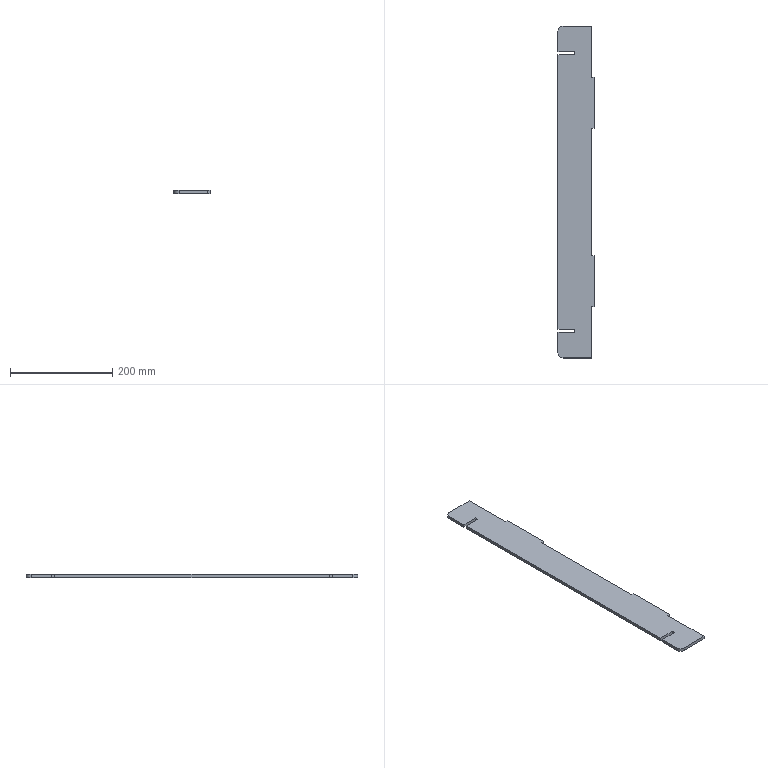Part | SolidWorks | features FlatPattern 1, SMBaseFlange 1, SheetMetal 1 | 1 solid | 24 faces | box 70.5 x 650 x 6 mm | volume 257466 mm3 | plane 22 | cylinder 2 | commonest cylinder face diameters 20 x2
STEP:
#1=CARTESIAN_POINT('',(549.5,252.363,0.));
#2=VERTEX_POINT('',#1);
#3=CARTESIAN_POINT('',(549.5,352.363,0.));
#4=VERTEX_POINT('',#3);
#5=CARTESIAN_POINT('',(549.5,352.363,0.));
#6=DIRECTION('',(0.,1.,0.));
#7=VECTOR('',#6,1000.);
#8=LINE('',#5,#7);
#9=EDGE_CURVE('',#2,#4,#8,.T.);
#10=ORIENTED_EDGE('',*,*,#9,.F.);
#11=CARTESIAN_POINT('',(549.5,252.363,-6.));
#12=VERTEX_POINT('',#11);
#13=CARTESIAN_POINT('',(549.5,252.363,-6.));
#14=DIRECTION('',(0.,0.,1.));
#15=VECTOR('',#14,1000.);
#16=LINE('',#13,#15);
#17=EDGE_CURVE('',#12,#2,#16,.T.);
#18=ORIENTED_EDGE('',*,*,#17,.F.);
#19=CARTESIAN_POINT('',(549.5,352.363,-6.));
#20=VERTEX_POINT('',#19);
#21=CARTESIAN_POINT('',(549.5,352.363,-6.));
#22=DIRECTION('',(0.,1.,0.));
#23=VECTOR('',#22,1000.);
#24=LINE('',#21,#23);
#25=EDGE_CURVE('',#12,#20,#24,.T.);
#26=ORIENTED_EDGE('',*,*,#25,.T.);
#27=CARTESIAN_POINT('',(549.5,352.363,-6.));
#28=DIRECTION('',(0.,0.,1.));
#29=VECTOR('',#28,1000.);
#30=LINE('',#27,#29);
#31=EDGE_CURVE('',#20,#4,#30,.T.);
#32=ORIENTED_EDGE('',*,*,#31,.T.);
#33=EDGE_LOOP('',(#10,#18,#26,#32));
#34=FACE_OUTER_BOUND('',#33,.T.);
#35=CARTESIAN_POINT('',(549.5,352.363,-6.));
#36=DIRECTION('',(1.,0.,0.));
#37=DIRECTION('',(0.,0.,-1.));
#38=AXIS2_PLACEMENT_3D('',#35,#36,#37);
#39=PLANE('',#38);
#40=ADVANCED_FACE('',(#34),#39,.T.);
#41=CARTESIAN_POINT('',(555.,252.363,0.));
#42=VERTEX_POINT('',#41);
#43=CARTESIAN_POINT('',(549.5,252.363,0.));
#44=DIRECTION('',(-1.,0.,0.));
#45=VECTOR('',#44,1000.);
#46=LINE('',#43,#45);
#47=EDGE_CURVE('',#42,#2,#46,.T.);
#48=ORIENTED_EDGE('',*,*,#47,.F.);
#49=CARTESIAN_POINT('',(555.,252.363,-6.));
#50=VERTEX_POINT('',#49);
#51=CARTESIAN_POINT('',(555.,252.363,-6.));
#52=DIRECTION('',(0.,0.,1.));
#53=VECTOR('',#52,1000.);
#54=LINE('',#51,#53);
#55=EDGE_CURVE('',#50,#42,#54,.T.);
#56=ORIENTED_EDGE('',*,*,#55,.F.);
#57=CARTESIAN_POINT('',(549.5,252.363,-6.));
#58=DIRECTION('',(-1.,0.,0.));
#59=VECTOR('',#58,1000.);
#60=LINE('',#57,#59);
#61=EDGE_CURVE('',#50,#12,#60,.T.);
#62=ORIENTED_EDGE('',*,*,#61,.T.);
#63=ORIENTED_EDGE('',*,*,#17,.T.);
#64=EDGE_LOOP('',(#48,#56,#62,#63));
#65=FACE_OUTER_BOUND('',#64,.T.);
#66=CARTESIAN_POINT('',(549.5,252.363,-6.));
#67=DIRECTION('',(0.,1.,0.));
#68=DIRECTION('',(0.,0.,1.));
#69=AXIS2_PLACEMENT_3D('',#66,#67,#68);
#70=PLANE('',#69);
#71=ADVANCED_FACE('',(#65),#70,.T.);
#72=CARTESIAN_POINT('',(555.,152.363,0.));
#73=VERTEX_POINT('',#72);
#74=CARTESIAN_POINT('',(555.,252.363,0.));
#75=DIRECTION('',(0.,1.,0.));
#76=VECTOR('',#75,1000.);
#77=LINE('',#74,#76);
#78=EDGE_CURVE('',#73,#42,#77,.T.);
#79=ORIENTED_EDGE('',*,*,#78,.F.);
#80=CARTESIAN_POINT('',(555.,152.363,-6.));
#81=VERTEX_POINT('',#80);
#82=CARTESIAN_POINT('',(555.,152.363,-6.));
#83=DIRECTION('',(0.,0.,1.));
#84=VECTOR('',#83,1000.);
#85=LINE('',#82,#84);
#86=EDGE_CURVE('',#81,#73,#85,.T.);
#87=ORIENTED_EDGE('',*,*,#86,.F.);
#88=CARTESIAN_POINT('',(555.,252.363,-6.));
#89=DIRECTION('',(0.,1.,0.));
#90=VECTOR('',#89,1000.);
#91=LINE('',#88,#90);
#92=EDGE_CURVE('',#81,#50,#91,.T.);
#93=ORIENTED_EDGE('',*,*,#92,.T.);
#94=ORIENTED_EDGE('',*,*,#55,.T.);
#95=EDGE_LOOP('',(#79,#87,#93,#94));
#96=FACE_OUTER_BOUND('',#95,.T.);
#97=CARTESIAN_POINT('',(555.,252.363,-6.));
#98=DIRECTION('',(1.,0.,0.));
#99=DIRECTION('',(0.,0.,-1.));
#100=AXIS2_PLACEMENT_3D('',#97,#98,#99);
#101=PLANE('',#100);
#102=ADVANCED_FACE('',(#96),#101,.T.);
#103=CARTESIAN_POINT('',(549.5,152.363,0.));
#104=VERTEX_POINT('',#103);
#105=CARTESIAN_POINT('',(555.,152.363,0.));
#106=DIRECTION('',(1.,0.,0.));
#107=VECTOR('',#106,1000.);
#108=LINE('',#105,#107);
#109=EDGE_CURVE('',#104,#73,#108,.T.);
#110=ORIENTED_EDGE('',*,*,#109,.F.);
#111=CARTESIAN_POINT('',(549.5,152.363,-6.));
#112=VERTEX_POINT('',#111);
#113=CARTESIAN_POINT('',(549.5,152.363,-6.));
#114=DIRECTION('',(0.,0.,1.));
#115=VECTOR('',#114,1000.);
#116=LINE('',#113,#115);
#117=EDGE_CURVE('',#112,#104,#116,.T.);
#118=ORIENTED_EDGE('',*,*,#117,.F.);
#119=CARTESIAN_POINT('',(555.,152.363,-6.));
#120=DIRECTION('',(1.,0.,0.));
#121=VECTOR('',#120,1000.);
#122=LINE('',#119,#121);
#123=EDGE_CURVE('',#112,#81,#122,.T.);
#124=ORIENTED_EDGE('',*,*,#123,.T.);
#125=ORIENTED_EDGE('',*,*,#86,.T.);
#126=EDGE_LOOP('',(#110,#118,#124,#125));
#127=FACE_OUTER_BOUND('',#126,.T.);
#128=CARTESIAN_POINT('',(555.,152.363,-6.));
#129=DIRECTION('',(0.,-1.,0.));
#130=DIRECTION('',(0.,0.,-1.));
#131=AXIS2_PLACEMENT_3D('',#128,#129,#130);
#132=PLANE('',#131);
#133=ADVANCED_FACE('',(#127),#132,.T.);
#134=CARTESIAN_POINT('',(549.5,-97.637,0.));
#135=VERTEX_POINT('',#134);
#136=CARTESIAN_POINT('',(549.5,152.363,0.));
#137=DIRECTION('',(0.,1.,0.));
#138=VECTOR('',#137,1000.);
#139=LINE('',#136,#138);
#140=EDGE_CURVE('',#135,#104,#139,.T.);
#141=ORIENTED_EDGE('',*,*,#140,.F.);
#142=CARTESIAN_POINT('',(549.5,-97.637,-6.));
#143=VERTEX_POINT('',#142);
#144=CARTESIAN_POINT('',(549.5,-97.637,-6.));
#145=DIRECTION('',(0.,0.,1.));
#146=VECTOR('',#145,1000.);
#147=LINE('',#144,#146);
#148=EDGE_CURVE('',#143,#135,#147,.T.);
#149=ORIENTED_EDGE('',*,*,#148,.F.);
#150=CARTESIAN_POINT('',(549.5,152.363,-6.));
#151=DIRECTION('',(0.,1.,0.));
#152=VECTOR('',#151,1000.);
#153=LINE('',#150,#152);
#154=EDGE_CURVE('',#143,#112,#153,.T.);
#155=ORIENTED_EDGE('',*,*,#154,.T.);
#156=ORIENTED_EDGE('',*,*,#117,.T.);
#157=EDGE_LOOP('',(#141,#149,#155,#156));
#158=FACE_OUTER_BOUND('',#157,.T.);
#159=CARTESIAN_POINT('',(549.5,152.363,-6.));
#160=DIRECTION('',(1.,0.,0.));
#161=DIRECTION('',(0.,0.,-1.));
#162=AXIS2_PLACEMENT_3D('',#159,#160,#161);
#163=PLANE('',#162);
#164=ADVANCED_FACE('',(#158),#163,.T.);
#165=CARTESIAN_POINT('',(555.,-97.637,0.));
#166=VERTEX_POINT('',#165);
#167=CARTESIAN_POINT('',(555.,-97.637,0.));
#168=DIRECTION('',(-1.,0.,0.));
#169=VECTOR('',#168,1000.);
#170=LINE('',#167,#169);
#171=EDGE_CURVE('',#166,#135,#170,.T.);
#172=ORIENTED_EDGE('',*,*,#171,.F.);
#173=CARTESIAN_POINT('',(555.,-97.637,-6.));
#174=VERTEX_POINT('',#173);
#175=CARTESIAN_POINT('',(555.,-97.637,-6.));
#176=DIRECTION('',(0.,0.,1.));
#177=VECTOR('',#176,1000.);
#178=LINE('',#175,#177);
#179=EDGE_CURVE('',#174,#166,#178,.T.);
#180=ORIENTED_EDGE('',*,*,#179,.F.);
#181=CARTESIAN_POINT('',(555.,-97.637,-6.));
#182=DIRECTION('',(-1.,0.,0.));
#183=VECTOR('',#182,1000.);
#184=LINE('',#181,#183);
#185=EDGE_CURVE('',#174,#143,#184,.T.);
#186=ORIENTED_EDGE('',*,*,#185,.T.);
#187=ORIENTED_EDGE('',*,*,#148,.T.);
#188=EDGE_LOOP('',(#172,#180,#186,#187));
#189=FACE_OUTER_BOUND('',#188,.T.);
#190=CARTESIAN_POINT('',(555.,-97.637,-6.));
#191=DIRECTION('',(0.,1.,0.));
#192=DIRECTION('',(-1.,0.,0.));
#193=AXIS2_PLACEMENT_3D('',#190,#191,#192);
#194=PLANE('',#193);
#195=ADVANCED_FACE('',(#189),#194,.T.);
#196=CARTESIAN_POINT('',(555.,-197.637,0.));
#197=VERTEX_POINT('',#196);
#198=CARTESIAN_POINT('',(555.,-197.637,0.));
#199=DIRECTION('',(0.,1.,0.));
#200=VECTOR('',#199,1000.);
#201=LINE('',#198,#200);
#202=EDGE_CURVE('',#197,#166,#201,.T.);
#203=ORIENTED_EDGE('',*,*,#202,.F.);
#204=CARTESIAN_POINT('',(555.,-197.637,-6.));
#205=VERTEX_POINT('',#204);
#206=CARTESIAN_POINT('',(555.,-197.637,-6.));
#207=DIRECTION('',(0.,0.,1.));
#208=VECTOR('',#207,1000.);
#209=LINE('',#206,#208);
#210=EDGE_CURVE('',#205,#197,#209,.T.);
#211=ORIENTED_EDGE('',*,*,#210,.F.);
#212=CARTESIAN_POINT('',(555.,-197.637,-6.));
#213=DIRECTION('',(0.,1.,0.));
#214=VECTOR('',#213,1000.);
#215=LINE('',#212,#214);
#216=EDGE_CURVE('',#205,#174,#215,.T.);
#217=ORIENTED_EDGE('',*,*,#216,.T.);
#218=ORIENTED_EDGE('',*,*,#179,.T.);
#219=EDGE_LOOP('',(#203,#211,#217,#218));
#220=FACE_OUTER_BOUND('',#219,.T.);
#221=CARTESIAN_POINT('',(555.,-197.637,-6.));
#222=DIRECTION('',(1.,0.,0.));
#223=DIRECTION('',(0.,1.,0.));
#224=AXIS2_PLACEMENT_3D('',#221,#222,#223);
#225=PLANE('',#224);
#226=ADVANCED_FACE('',(#220),#225,.T.);
#227=CARTESIAN_POINT('',(549.5,-197.637,0.));
#228=VERTEX_POINT('',#227);
#229=CARTESIAN_POINT('',(549.5,-197.637,0.));
#230=DIRECTION('',(1.,0.,0.));
#231=VECTOR('',#230,1000.);
#232=LINE('',#229,#231);
#233=EDGE_CURVE('',#228,#197,#232,.T.);
#234=ORIENTED_EDGE('',*,*,#233,.F.);
#235=CARTESIAN_POINT('',(549.5,-197.637,-6.));
#236=VERTEX_POINT('',#235);
#237=CARTESIAN_POINT('',(549.5,-197.637,-6.));
#238=DIRECTION('',(0.,0.,1.));
#239=VECTOR('',#238,1000.);
#240=LINE('',#237,#239);
#241=EDGE_CURVE('',#236,#228,#240,.T.);
#242=ORIENTED_EDGE('',*,*,#241,.F.);
#243=CARTESIAN_POINT('',(549.5,-197.637,-6.));
#244=DIRECTION('',(1.,0.,0.));
#245=VECTOR('',#244,1000.);
#246=LINE('',#243,#245);
#247=EDGE_CURVE('',#236,#205,#246,.T.);
#248=ORIENTED_EDGE('',*,*,#247,.T.);
#249=ORIENTED_EDGE('',*,*,#210,.T.);
#250=EDGE_LOOP('',(#234,#242,#248,#249));
#251=FACE_OUTER_BOUND('',#250,.T.);
#252=CARTESIAN_POINT('',(549.5,-197.637,-6.));
#253=DIRECTION('',(0.,-1.,0.));
#254=DIRECTION('',(0.,0.,-1.));
#255=AXIS2_PLACEMENT_3D('',#252,#253,#254);
#256=PLANE('',#255);
#257=ADVANCED_FACE('',(#251),#256,.T.);
#258=CARTESIAN_POINT('',(549.5,-297.637,0.));
#259=VERTEX_POINT('',#258);
#260=CARTESIAN_POINT('',(549.5,-197.637,0.));
#261=DIRECTION('',(0.,1.,0.));
#262=VECTOR('',#261,1000.);
#263=LINE('',#260,#262);
#264=EDGE_CURVE('',#259,#228,#263,.T.);
#265=ORIENTED_EDGE('',*,*,#264,.F.);
#266=CARTESIAN_POINT('',(549.5,-297.637,-6.));
#267=VERTEX_POINT('',#266);
#268=CARTESIAN_POINT('',(549.5,-297.637,-6.));
#269=DIRECTION('',(0.,0.,1.));
#270=VECTOR('',#269,1000.);
#271=LINE('',#268,#270);
#272=EDGE_CURVE('',#267,#259,#271,.T.);
#273=ORIENTED_EDGE('',*,*,#272,.F.);
#274=CARTESIAN_POINT('',(549.5,-197.637,-6.));
#275=DIRECTION('',(0.,1.,0.));
#276=VECTOR('',#275,1000.);
#277=LINE('',#274,#276);
#278=EDGE_CURVE('',#267,#236,#277,.T.);
#279=ORIENTED_EDGE('',*,*,#278,.T.);
#280=ORIENTED_EDGE('',*,*,#241,.T.);
#281=EDGE_LOOP('',(#265,#273,#279,#280));
#282=FACE_OUTER_BOUND('',#281,.T.);
#283=CARTESIAN_POINT('',(549.5,-197.637,-6.));
#284=DIRECTION('',(1.,0.,0.));
#285=DIRECTION('',(0.,1.,0.));
#286=AXIS2_PLACEMENT_3D('',#283,#284,#285);
#287=PLANE('',#286);
#288=ADVANCED_FACE('',(#282),#287,.T.);
#289=CARTESIAN_POINT('',(494.5,-297.637,0.));
#290=VERTEX_POINT('',#289);
#291=CARTESIAN_POINT('',(549.5,-297.637,0.));
#292=DIRECTION('',(1.,0.,0.));
#293=VECTOR('',#292,1000.);
#294=LINE('',#291,#293);
#295=EDGE_CURVE('',#290,#259,#294,.T.);
#296=ORIENTED_EDGE('',*,*,#295,.F.);
#297=CARTESIAN_POINT('',(494.5,-297.637,-6.));
#298=VERTEX_POINT('',#297);
#299=CARTESIAN_POINT('',(494.5,-297.637,-6.));
#300=DIRECTION('',(0.,0.,1.));
#301=VECTOR('',#300,1000.);
#302=LINE('',#299,#301);
#303=EDGE_CURVE('',#298,#290,#302,.T.);
#304=ORIENTED_EDGE('',*,*,#303,.F.);
#305=CARTESIAN_POINT('',(549.5,-297.637,-6.));
#306=DIRECTION('',(1.,0.,0.));
#307=VECTOR('',#306,1000.);
#308=LINE('',#305,#307);
#309=EDGE_CURVE('',#298,#267,#308,.T.);
#310=ORIENTED_EDGE('',*,*,#309,.T.);
#311=ORIENTED_EDGE('',*,*,#272,.T.);
#312=EDGE_LOOP('',(#296,#304,#310,#311));
#313=FACE_OUTER_BOUND('',#312,.T.);
#314=CARTESIAN_POINT('',(549.5,-297.637,-6.));
#315=DIRECTION('',(0.,-1.,0.));
#316=DIRECTION('',(0.,0.,-1.));
#317=AXIS2_PLACEMENT_3D('',#314,#315,#316);
#318=PLANE('',#317);
#319=ADVANCED_FACE('',(#313),#318,.T.);
#320=CARTESIAN_POINT('',(484.5,-287.637,0.));
#321=VERTEX_POINT('',#320);
#322=CARTESIAN_POINT('',(494.5,-287.637,0.));
#323=DIRECTION('',(0.,0.,1.));
#324=DIRECTION('',(-1.,0.,0.));
#325=AXIS2_PLACEMENT_3D('',#322,#323,#324);
#326=CIRCLE('',#325,10.);
#327=EDGE_CURVE('',#321,#290,#326,.T.);
#328=ORIENTED_EDGE('',*,*,#327,.F.);
#329=CARTESIAN_POINT('',(484.5,-287.637,-6.));
#330=VERTEX_POINT('',#329);
#331=CARTESIAN_POINT('',(484.5,-287.637,-6.));
#332=DIRECTION('',(0.,0.,1.));
#333=VECTOR('',#332,1000.);
#334=LINE('',#331,#333);
#335=EDGE_CURVE('',#330,#321,#334,.T.);
#336=ORIENTED_EDGE('',*,*,#335,.F.);
#337=CARTESIAN_POINT('',(494.5,-287.637,-6.));
#338=DIRECTION('',(0.,0.,1.));
#339=DIRECTION('',(-1.,0.,0.));
#340=AXIS2_PLACEMENT_3D('',#337,#338,#339);
#341=CIRCLE('',#340,10.);
#342=EDGE_CURVE('',#330,#298,#341,.T.);
#343=ORIENTED_EDGE('',*,*,#342,.T.);
#344=ORIENTED_EDGE('',*,*,#303,.T.);
#345=EDGE_LOOP('',(#328,#336,#343,#344));
#346=FACE_OUTER_BOUND('',#345,.T.);
#347=CARTESIAN_POINT('',(494.5,-287.637,-6.));
#348=DIRECTION('',(0.,0.,1.));
#349=DIRECTION('',(1.,0.,0.));
#350=AXIS2_PLACEMENT_3D('',#347,#348,#349);
#351=CYLINDRICAL_SURFACE('',#350,10.);
#352=ADVANCED_FACE('',(#346),#351,.T.);
#353=CARTESIAN_POINT('',(484.5,-247.637,0.));
#354=VERTEX_POINT('',#353);
#355=CARTESIAN_POINT('',(484.5,-247.637,0.));
#356=DIRECTION('',(0.,-1.,0.));
#357=VECTOR('',#356,1000.);
#358=LINE('',#355,#357);
#359=EDGE_CURVE('',#354,#321,#358,.T.);
#360=ORIENTED_EDGE('',*,*,#359,.F.);
#361=CARTESIAN_POINT('',(484.5,-247.637,-6.));
#362=VERTEX_POINT('',#361);
#363=CARTESIAN_POINT('',(484.5,-247.637,-6.));
#364=DIRECTION('',(0.,0.,1.));
#365=VECTOR('',#364,1000.);
#366=LINE('',#363,#365);
#367=EDGE_CURVE('',#362,#354,#366,.T.);
#368=ORIENTED_EDGE('',*,*,#367,.F.);
#369=CARTESIAN_POINT('',(484.5,-247.637,-6.));
#370=DIRECTION('',(0.,-1.,0.));
#371=VECTOR('',#370,1000.);
#372=LINE('',#369,#371);
#373=EDGE_CURVE('',#362,#330,#372,.T.);
#374=ORIENTED_EDGE('',*,*,#373,.T.);
#375=ORIENTED_EDGE('',*,*,#335,.T.);
#376=EDGE_LOOP('',(#360,#368,#374,#375));
#377=FACE_OUTER_BOUND('',#376,.T.);
#378=CARTESIAN_POINT('',(484.5,-247.637,-6.));
#379=DIRECTION('',(-1.,0.,0.));
#380=DIRECTION('',(0.,-1.,0.));
#381=AXIS2_PLACEMENT_3D('',#378,#379,#380);
#382=PLANE('',#381);
#383=ADVANCED_FACE('',(#377),#382,.T.);
#384=CARTESIAN_POINT('',(517.5,-247.637,0.));
#385=VERTEX_POINT('',#384);
#386=CARTESIAN_POINT('',(517.5,-247.637,0.));
#387=DIRECTION('',(-1.,0.,0.));
#388=VECTOR('',#387,1000.);
#389=LINE('',#386,#388);
#390=EDGE_CURVE('',#385,#354,#389,.T.);
#391=ORIENTED_EDGE('',*,*,#390,.F.);
#392=CARTESIAN_POINT('',(517.5,-247.637,-6.));
#393=VERTEX_POINT('',#392);
#394=CARTESIAN_POINT('',(517.5,-247.637,-6.));
#395=DIRECTION('',(0.,0.,1.));
#396=VECTOR('',#395,1000.);
#397=LINE('',#394,#396);
#398=EDGE_CURVE('',#393,#385,#397,.T.);
#399=ORIENTED_EDGE('',*,*,#398,.F.);
#400=CARTESIAN_POINT('',(517.5,-247.637,-6.));
#401=DIRECTION('',(-1.,0.,0.));
#402=VECTOR('',#401,1000.);
#403=LINE('',#400,#402);
#404=EDGE_CURVE('',#393,#362,#403,.T.);
#405=ORIENTED_EDGE('',*,*,#404,.T.);
#406=ORIENTED_EDGE('',*,*,#367,.T.);
#407=EDGE_LOOP('',(#391,#399,#405,#406));
#408=FACE_OUTER_BOUND('',#407,.T.);
#409=CARTESIAN_POINT('',(517.5,-247.637,-6.));
#410=DIRECTION('',(0.,1.,0.));
#411=DIRECTION('',(0.,0.,1.));
#412=AXIS2_PLACEMENT_3D('',#409,#410,#411);
#413=PLANE('',#412);
#414=ADVANCED_FACE('',(#408),#413,.T.);
#415=CARTESIAN_POINT('',(517.5,-241.637,0.));
#416=VERTEX_POINT('',#415);
#417=CARTESIAN_POINT('',(517.5,-241.637,0.));
#418=DIRECTION('',(0.,-1.,0.));
#419=VECTOR('',#418,1000.);
#420=LINE('',#417,#419);
#421=EDGE_CURVE('',#416,#385,#420,.T.);
#422=ORIENTED_EDGE('',*,*,#421,.F.);
#423=CARTESIAN_POINT('',(517.5,-241.637,-6.));
#424=VERTEX_POINT('',#423);
#425=CARTESIAN_POINT('',(517.5,-241.637,-6.));
#426=DIRECTION('',(0.,0.,1.));
#427=VECTOR('',#426,1000.);
#428=LINE('',#425,#427);
#429=EDGE_CURVE('',#424,#416,#428,.T.);
#430=ORIENTED_EDGE('',*,*,#429,.F.);
#431=CARTESIAN_POINT('',(517.5,-241.637,-6.));
#432=DIRECTION('',(0.,-1.,0.));
#433=VECTOR('',#432,1000.);
#434=LINE('',#431,#433);
#435=EDGE_CURVE('',#424,#393,#434,.T.);
#436=ORIENTED_EDGE('',*,*,#435,.T.);
#437=ORIENTED_EDGE('',*,*,#398,.T.);
#438=EDGE_LOOP('',(#422,#430,#436,#437));
#439=FACE_OUTER_BOUND('',#438,.T.);
#440=CARTESIAN_POINT('',(517.5,-241.637,-6.));
#441=DIRECTION('',(-1.,0.,0.));
#442=DIRECTION('',(0.,0.,1.));
#443=AXIS2_PLACEMENT_3D('',#440,#441,#442);
#444=PLANE('',#443);
#445=ADVANCED_FACE('',(#439),#444,.T.);
#446=CARTESIAN_POINT('',(484.5,-241.637,0.));
#447=VERTEX_POINT('',#446);
#448=CARTESIAN_POINT('',(484.5,-241.637,0.));
#449=DIRECTION('',(1.,0.,0.));
#450=VECTOR('',#449,1000.);
#451=LINE('',#448,#450);
#452=EDGE_CURVE('',#447,#416,#451,.T.);
#453=ORIENTED_EDGE('',*,*,#452,.F.);
#454=CARTESIAN_POINT('',(484.5,-241.637,-6.));
#455=VERTEX_POINT('',#454);
#456=CARTESIAN_POINT('',(484.5,-241.637,-6.));
#457=DIRECTION('',(0.,0.,1.));
#458=VECTOR('',#457,1000.);
#459=LINE('',#456,#458);
#460=EDGE_CURVE('',#455,#447,#459,.T.);
#461=ORIENTED_EDGE('',*,*,#460,.F.);
#462=CARTESIAN_POINT('',(484.5,-241.637,-6.));
#463=DIRECTION('',(1.,0.,0.));
#464=VECTOR('',#463,1000.);
#465=LINE('',#462,#464);
#466=EDGE_CURVE('',#455,#424,#465,.T.);
#467=ORIENTED_EDGE('',*,*,#466,.T.);
#468=ORIENTED_EDGE('',*,*,#429,.T.);
#469=EDGE_LOOP('',(#453,#461,#467,#468));
#470=FACE_OUTER_BOUND('',#469,.T.);
#471=CARTESIAN_POINT('',(484.5,-241.637,-6.));
#472=DIRECTION('',(0.,-1.,0.));
#473=DIRECTION('',(0.,0.,-1.));
#474=AXIS2_PLACEMENT_3D('',#471,#472,#473);
#475=PLANE('',#474);
#476=ADVANCED_FACE('',(#470),#475,.T.);
#477=CARTESIAN_POINT('',(484.5,296.363,0.));
#478=VERTEX_POINT('',#477);
#479=CARTESIAN_POINT('',(484.5,296.363,0.));
#480=DIRECTION('',(0.,-1.,0.));
#481=VECTOR('',#480,1000.);
#482=LINE('',#479,#481);
#483=EDGE_CURVE('',#478,#447,#482,.T.);
#484=ORIENTED_EDGE('',*,*,#483,.F.);
#485=CARTESIAN_POINT('',(484.5,296.363,-6.));
#486=VERTEX_POINT('',#485);
#487=CARTESIAN_POINT('',(484.5,296.363,-6.));
#488=DIRECTION('',(0.,0.,1.));
#489=VECTOR('',#488,1000.);
#490=LINE('',#487,#489);
#491=EDGE_CURVE('',#486,#478,#490,.T.);
#492=ORIENTED_EDGE('',*,*,#491,.F.);
#493=CARTESIAN_POINT('',(484.5,296.363,-6.));
#494=DIRECTION('',(0.,-1.,0.));
#495=VECTOR('',#494,1000.);
#496=LINE('',#493,#495);
#497=EDGE_CURVE('',#486,#455,#496,.T.);
#498=ORIENTED_EDGE('',*,*,#497,.T.);
#499=ORIENTED_EDGE('',*,*,#460,.T.);
#500=EDGE_LOOP('',(#484,#492,#498,#499));
#501=FACE_OUTER_BOUND('',#500,.T.);
#502=CARTESIAN_POINT('',(484.5,296.363,-6.));
#503=DIRECTION('',(-1.,0.,0.));
#504=DIRECTION('',(0.,-1.,0.));
#505=AXIS2_PLACEMENT_3D('',#502,#503,#504);
#506=PLANE('',#505);
#507=ADVANCED_FACE('',(#501),#506,.T.);
#508=CARTESIAN_POINT('',(517.5,296.363,0.));
#509=VERTEX_POINT('',#508);
#510=CARTESIAN_POINT('',(517.5,296.363,0.));
#511=DIRECTION('',(-1.,0.,0.));
#512=VECTOR('',#511,1000.);
#513=LINE('',#510,#512);
#514=EDGE_CURVE('',#509,#478,#513,.T.);
#515=ORIENTED_EDGE('',*,*,#514,.F.);
#516=CARTESIAN_POINT('',(517.5,296.363,-6.));
#517=VERTEX_POINT('',#516);
#518=CARTESIAN_POINT('',(517.5,296.363,-6.));
#519=DIRECTION('',(0.,0.,1.));
#520=VECTOR('',#519,1000.);
#521=LINE('',#518,#520);
#522=EDGE_CURVE('',#517,#509,#521,.T.);
#523=ORIENTED_EDGE('',*,*,#522,.F.);
#524=CARTESIAN_POINT('',(517.5,296.363,-6.));
#525=DIRECTION('',(-1.,0.,0.));
#526=VECTOR('',#525,1000.);
#527=LINE('',#524,#526);
#528=EDGE_CURVE('',#517,#486,#527,.T.);
#529=ORIENTED_EDGE('',*,*,#528,.T.);
#530=ORIENTED_EDGE('',*,*,#491,.T.);
#531=EDGE_LOOP('',(#515,#523,#529,#530));
#532=FACE_OUTER_BOUND('',#531,.T.);
#533=CARTESIAN_POINT('',(517.5,296.363,-6.));
#534=DIRECTION('',(0.,1.,0.));
#535=DIRECTION('',(0.,0.,1.));
#536=AXIS2_PLACEMENT_3D('',#533,#534,#535);
#537=PLANE('',#536);
#538=ADVANCED_FACE('',(#532),#537,.T.);
#539=CARTESIAN_POINT('',(517.5,302.363,0.));
#540=VERTEX_POINT('',#539);
#541=CARTESIAN_POINT('',(517.5,302.363,0.));
#542=DIRECTION('',(0.,-1.,0.));
#543=VECTOR('',#542,1000.);
#544=LINE('',#541,#543);
#545=EDGE_CURVE('',#540,#509,#544,.T.);
#546=ORIENTED_EDGE('',*,*,#545,.F.);
#547=CARTESIAN_POINT('',(517.5,302.363,-6.));
#548=VERTEX_POINT('',#547);
#549=CARTESIAN_POINT('',(517.5,302.363,-6.));
#550=DIRECTION('',(0.,0.,1.));
#551=VECTOR('',#550,1000.);
#552=LINE('',#549,#551);
#553=EDGE_CURVE('',#548,#540,#552,.T.);
#554=ORIENTED_EDGE('',*,*,#553,.F.);
#555=CARTESIAN_POINT('',(517.5,302.363,-6.));
#556=DIRECTION('',(0.,-1.,0.));
#557=VECTOR('',#556,1000.);
#558=LINE('',#555,#557);
#559=EDGE_CURVE('',#548,#517,#558,.T.);
#560=ORIENTED_EDGE('',*,*,#559,.T.);
#561=ORIENTED_EDGE('',*,*,#522,.T.);
#562=EDGE_LOOP('',(#546,#554,#560,#561));
#563=FACE_OUTER_BOUND('',#562,.T.);
#564=CARTESIAN_POINT('',(517.5,302.363,-6.));
#565=DIRECTION('',(-1.,0.,0.));
#566=DIRECTION('',(0.,0.,1.));
#567=AXIS2_PLACEMENT_3D('',#564,#565,#566);
#568=PLANE('',#567);
#569=ADVANCED_FACE('',(#563),#568,.T.);
#570=CARTESIAN_POINT('',(484.5,302.363,0.));
#571=VERTEX_POINT('',#570);
#572=CARTESIAN_POINT('',(484.5,302.363,0.));
#573=DIRECTION('',(1.,0.,0.));
#574=VECTOR('',#573,1000.);
#575=LINE('',#572,#574);
#576=EDGE_CURVE('',#571,#540,#575,.T.);
#577=ORIENTED_EDGE('',*,*,#576,.F.);
#578=CARTESIAN_POINT('',(484.5,302.363,-6.));
#579=VERTEX_POINT('',#578);
#580=CARTESIAN_POINT('',(484.5,302.363,-6.));
#581=DIRECTION('',(0.,0.,1.));
#582=VECTOR('',#581,1000.);
#583=LINE('',#580,#582);
#584=EDGE_CURVE('',#579,#571,#583,.T.);
#585=ORIENTED_EDGE('',*,*,#584,.F.);
#586=CARTESIAN_POINT('',(484.5,302.363,-6.));
#587=DIRECTION('',(1.,0.,0.));
#588=VECTOR('',#587,1000.);
#589=LINE('',#586,#588);
#590=EDGE_CURVE('',#579,#548,#589,.T.);
#591=ORIENTED_EDGE('',*,*,#590,.T.);
#592=ORIENTED_EDGE('',*,*,#553,.T.);
#593=EDGE_LOOP('',(#577,#585,#591,#592));
#594=FACE_OUTER_BOUND('',#593,.T.);
#595=CARTESIAN_POINT('',(484.5,302.363,-6.));
#596=DIRECTION('',(0.,-1.,0.));
#597=DIRECTION('',(0.,0.,-1.));
#598=AXIS2_PLACEMENT_3D('',#595,#596,#597);
#599=PLANE('',#598);
#600=ADVANCED_FACE('',(#594),#599,.T.);
#601=CARTESIAN_POINT('',(484.5,342.363,0.));
#602=VERTEX_POINT('',#601);
#603=CARTESIAN_POINT('',(484.5,342.363,0.));
#604=DIRECTION('',(0.,-1.,0.));
#605=VECTOR('',#604,1000.);
#606=LINE('',#603,#605);
#607=EDGE_CURVE('',#602,#571,#606,.T.);
#608=ORIENTED_EDGE('',*,*,#607,.F.);
#609=CARTESIAN_POINT('',(484.5,342.363,-6.));
#610=VERTEX_POINT('',#609);
#611=CARTESIAN_POINT('',(484.5,342.363,-6.));
#612=DIRECTION('',(0.,0.,1.));
#613=VECTOR('',#612,1000.);
#614=LINE('',#611,#613);
#615=EDGE_CURVE('',#610,#602,#614,.T.);
#616=ORIENTED_EDGE('',*,*,#615,.F.);
#617=CARTESIAN_POINT('',(484.5,342.363,-6.));
#618=DIRECTION('',(0.,-1.,0.));
#619=VECTOR('',#618,1000.);
#620=LINE('',#617,#619);
#621=EDGE_CURVE('',#610,#579,#620,.T.);
#622=ORIENTED_EDGE('',*,*,#621,.T.);
#623=ORIENTED_EDGE('',*,*,#584,.T.);
#624=EDGE_LOOP('',(#608,#616,#622,#623));
#625=FACE_OUTER_BOUND('',#624,.T.);
#626=CARTESIAN_POINT('',(484.5,342.363,-6.));
#627=DIRECTION('',(-1.,0.,0.));
#628=DIRECTION('',(0.,-1.,0.));
#629=AXIS2_PLACEMENT_3D('',#626,#627,#628);
#630=PLANE('',#629);
#631=ADVANCED_FACE('',(#625),#630,.T.);
#632=CARTESIAN_POINT('',(494.5,352.363,0.));
#633=VERTEX_POINT('',#632);
#634=CARTESIAN_POINT('',(494.5,342.363,0.));
#635=DIRECTION('',(0.,0.,1.));
#636=DIRECTION('',(1.,0.,0.));
#637=AXIS2_PLACEMENT_3D('',#634,#635,#636);
#638=CIRCLE('',#637,10.);
#639=EDGE_CURVE('',#633,#602,#638,.T.);
#640=ORIENTED_EDGE('',*,*,#639,.F.);
#641=CARTESIAN_POINT('',(494.5,352.363,-6.));
#642=VERTEX_POINT('',#641);
#643=CARTESIAN_POINT('',(494.5,352.363,-6.));
#644=DIRECTION('',(0.,0.,1.));
#645=VECTOR('',#644,1000.);
#646=LINE('',#643,#645);
#647=EDGE_CURVE('',#642,#633,#646,.T.);
#648=ORIENTED_EDGE('',*,*,#647,.F.);
#649=CARTESIAN_POINT('',(494.5,342.363,-6.));
#650=DIRECTION('',(0.,0.,1.));
#651=DIRECTION('',(1.,0.,0.));
#652=AXIS2_PLACEMENT_3D('',#649,#650,#651);
#653=CIRCLE('',#652,10.);
#654=EDGE_CURVE('',#642,#610,#653,.T.);
#655=ORIENTED_EDGE('',*,*,#654,.T.);
#656=ORIENTED_EDGE('',*,*,#615,.T.);
#657=EDGE_LOOP('',(#640,#648,#655,#656));
#658=FACE_OUTER_BOUND('',#657,.T.);
#659=CARTESIAN_POINT('',(494.5,342.363,-6.));
#660=DIRECTION('',(0.,0.,1.));
#661=DIRECTION('',(1.,0.,0.));
#662=AXIS2_PLACEMENT_3D('',#659,#660,#661);
#663=CYLINDRICAL_SURFACE('',#662,10.);
#664=ADVANCED_FACE('',(#658),#663,.T.);
#665=CARTESIAN_POINT('',(549.5,352.363,0.));
#666=DIRECTION('',(-1.,0.,0.));
#667=VECTOR('',#666,1000.);
#668=LINE('',#665,#667);
#669=EDGE_CURVE('',#4,#633,#668,.T.);
#670=ORIENTED_EDGE('',*,*,#669,.F.);
#671=ORIENTED_EDGE('',*,*,#31,.F.);
#672=CARTESIAN_POINT('',(549.5,352.363,-6.));
#673=DIRECTION('',(-1.,0.,0.));
#674=VECTOR('',#673,1000.);
#675=LINE('',#672,#674);
#676=EDGE_CURVE('',#20,#642,#675,.T.);
#677=ORIENTED_EDGE('',*,*,#676,.T.);
#678=ORIENTED_EDGE('',*,*,#647,.T.);
#679=EDGE_LOOP('',(#670,#671,#677,#678));
#680=FACE_OUTER_BOUND('',#679,.T.);
#681=CARTESIAN_POINT('',(549.5,352.363,-6.));
#682=DIRECTION('',(0.,1.,0.));
#683=DIRECTION('',(0.,0.,1.));
#684=AXIS2_PLACEMENT_3D('',#681,#682,#683);
#685=PLANE('',#684);
#686=ADVANCED_FACE('',(#680),#685,.T.);
#687=ORIENTED_EDGE('',*,*,#25,.F.);
#688=ORIENTED_EDGE('',*,*,#61,.F.);
#689=ORIENTED_EDGE('',*,*,#92,.F.);
#690=ORIENTED_EDGE('',*,*,#123,.F.);
#691=ORIENTED_EDGE('',*,*,#154,.F.);
#692=ORIENTED_EDGE('',*,*,#185,.F.);
#693=ORIENTED_EDGE('',*,*,#216,.F.);
#694=ORIENTED_EDGE('',*,*,#247,.F.);
#695=ORIENTED_EDGE('',*,*,#278,.F.);
#696=ORIENTED_EDGE('',*,*,#309,.F.);
#697=ORIENTED_EDGE('',*,*,#342,.F.);
#698=ORIENTED_EDGE('',*,*,#373,.F.);
#699=ORIENTED_EDGE('',*,*,#404,.F.);
#700=ORIENTED_EDGE('',*,*,#435,.F.);
#701=ORIENTED_EDGE('',*,*,#466,.F.);
#702=ORIENTED_EDGE('',*,*,#497,.F.);
#703=ORIENTED_EDGE('',*,*,#528,.F.);
#704=ORIENTED_EDGE('',*,*,#559,.F.);
#705=ORIENTED_EDGE('',*,*,#590,.F.);
#706=ORIENTED_EDGE('',*,*,#621,.F.);
#707=ORIENTED_EDGE('',*,*,#654,.F.);
#708=ORIENTED_EDGE('',*,*,#676,.F.);
#709=EDGE_LOOP('',(#687,#688,#689,#690,#691,#692,#693,#694,#695,#696,#697,#698,#699,#700,#701,#702,#703,#704,#705,#706,#707,#708));
#710=FACE_OUTER_BOUND('',#709,.T.);
#711=CARTESIAN_POINT('',(494.5,-287.637,-6.));
#712=DIRECTION('',(0.,0.,-1.));
#713=DIRECTION('',(-1.,0.,0.));
#714=AXIS2_PLACEMENT_3D('',#711,#712,#713);
#715=PLANE('',#714);
#716=ADVANCED_FACE('',(#710),#715,.T.);
#717=ORIENTED_EDGE('',*,*,#9,.T.);
#718=ORIENTED_EDGE('',*,*,#669,.T.);
#719=ORIENTED_EDGE('',*,*,#639,.T.);
#720=ORIENTED_EDGE('',*,*,#607,.T.);
#721=ORIENTED_EDGE('',*,*,#576,.T.);
#722=ORIENTED_EDGE('',*,*,#545,.T.);
#723=ORIENTED_EDGE('',*,*,#514,.T.);
#724=ORIENTED_EDGE('',*,*,#483,.T.);
#725=ORIENTED_EDGE('',*,*,#452,.T.);
#726=ORIENTED_EDGE('',*,*,#421,.T.);
#727=ORIENTED_EDGE('',*,*,#390,.T.);
#728=ORIENTED_EDGE('',*,*,#359,.T.);
#729=ORIENTED_EDGE('',*,*,#327,.T.);
#730=ORIENTED_EDGE('',*,*,#295,.T.);
#731=ORIENTED_EDGE('',*,*,#264,.T.);
#732=ORIENTED_EDGE('',*,*,#233,.T.);
#733=ORIENTED_EDGE('',*,*,#202,.T.);
#734=ORIENTED_EDGE('',*,*,#171,.T.);
#735=ORIENTED_EDGE('',*,*,#140,.T.);
#736=ORIENTED_EDGE('',*,*,#109,.T.);
#737=ORIENTED_EDGE('',*,*,#78,.T.);
#738=ORIENTED_EDGE('',*,*,#47,.T.);
#739=EDGE_LOOP('',(#717,#718,#719,#720,#721,#722,#723,#724,#725,#726,#727,#728,#729,#730,#731,#732,#733,#734,#735,#736,#737,#738));
#740=FACE_OUTER_BOUND('',#739,.T.);
#741=CARTESIAN_POINT('',(494.5,-287.637,0.));
#742=DIRECTION('',(0.,0.,-1.));
#743=DIRECTION('',(-1.,0.,0.));
#744=AXIS2_PLACEMENT_3D('',#741,#742,#743);
#745=PLANE('',#744);
#746=ADVANCED_FACE('',(#740),#745,.F.);
#747=CLOSED_SHELL('',(#40,#71,#102,#133,#164,#195,#226,#257,#288,#319,#352,#383,#414,#445,#476,#507,#538,#569,#600,#631,#664,#686,#716,#746));
#748=MANIFOLD_SOLID_BREP('',#747);
#749=CARTESIAN_POINT('',(0.,0.,0.));
#750=DIRECTION('',(0.,0.,1.));
#751=DIRECTION('',(1.,0.,0.));
#752=AXIS2_PLACEMENT_3D('',#749,#750,#751);
#753=(LENGTH_UNIT()NAMED_UNIT(*)SI_UNIT(.MILLI.,.METRE.));
#754=UNCERTAINTY_MEASURE_WITH_UNIT(LENGTH_MEASURE(0.00001),#753,'','');
#755=(NAMED_UNIT(*)PLANE_ANGLE_UNIT()SI_UNIT($,.RADIAN.));
#756=(NAMED_UNIT(*)SI_UNIT($,.STERADIAN.)SOLID_ANGLE_UNIT());
#757=(GEOMETRIC_REPRESENTATION_CONTEXT(3)GLOBAL_UNCERTAINTY_ASSIGNED_CONTEXT((#754))GLOBAL_UNIT_ASSIGNED_CONTEXT((#753,#755,#756))REPRESENTATION_CONTEXT('',''));
#758=ADVANCED_BREP_SHAPE_REPRESENTATION('',(#748,#752),#757);